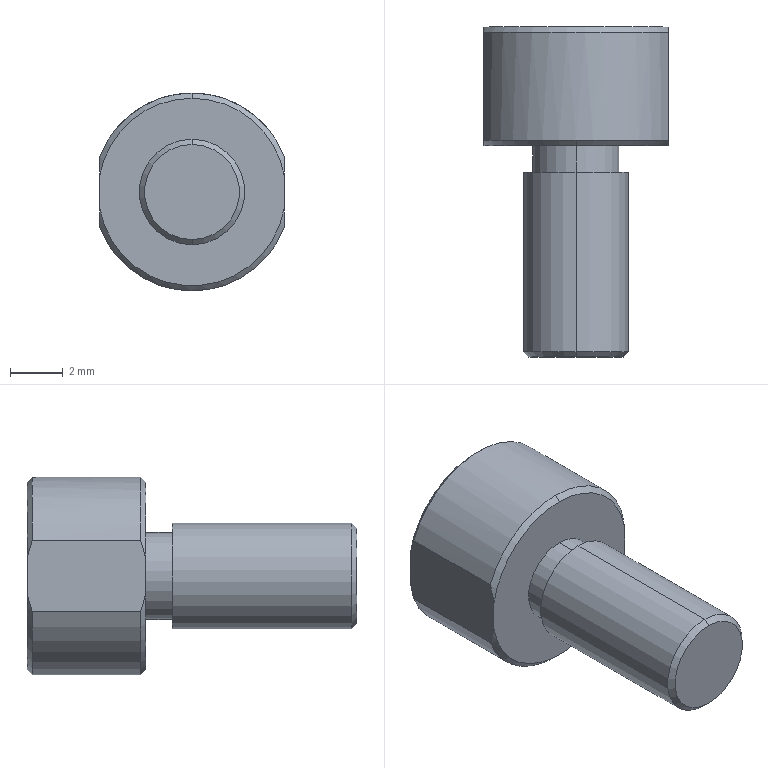Part | STEP file | PN_0021 fixture block | 1 solid | 21 faces | box 7 x 12.5 x 7.5 mm | volume 290.271 mm3 | cone 8 | cylinder 7 | plane 6 | commonest cylinder face diameters 7.5 x3 3.3 x2 4 x2